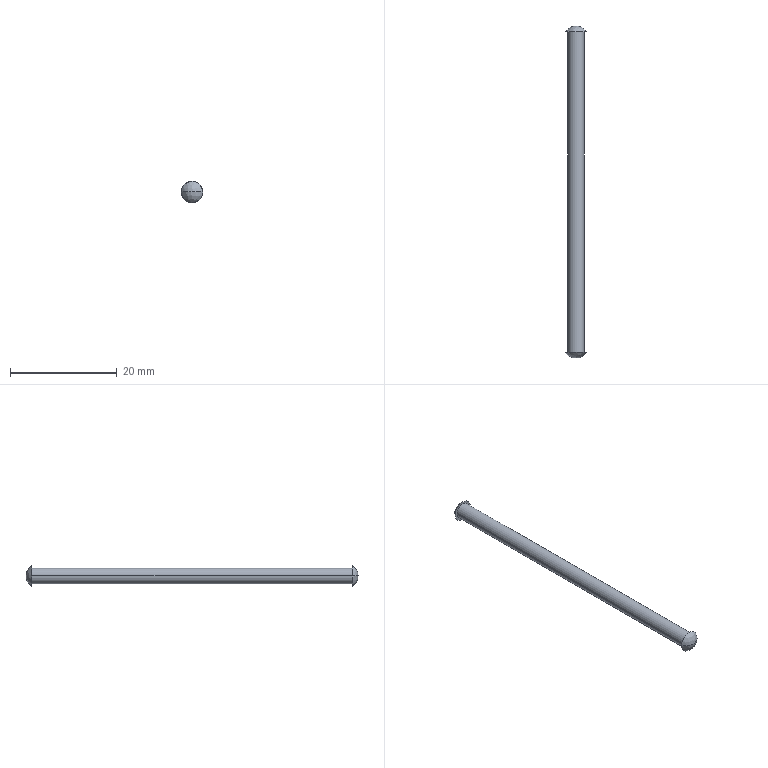Part | STEP file | Second B-1027-14 Shaft Part | 1 solid | 7 faces | box 4 x 62.171 x 4 mm | volume 439.342 mm3 | spline 3 | cylinder 2 | plane 2 | commonest cylinder face diameters 3 x2
STEP:
#1=CARTESIAN_POINT('',(-2.,-30.,0.));
#2=VERTEX_POINT('',#1);
#3=CARTESIAN_POINT('',(2.,-30.,0.));
#4=VERTEX_POINT('',#3);
#5=CARTESIAN_POINT('',(-2.,-30.,0.));
#6=CARTESIAN_POINT('',(-2.,-30.,-0.1321));
#7=CARTESIAN_POINT('',(-1.987,-30.,-0.262));
#8=CARTESIAN_POINT('',(-1.936,-30.,-0.5176));
#9=CARTESIAN_POINT('',(-1.898,-30.,-0.6446));
#10=CARTESIAN_POINT('',(-1.797,-30.,-0.8868));
#11=CARTESIAN_POINT('',(-1.736,-30.,-1.002));
#12=CARTESIAN_POINT('',(-1.591,-30.,-1.219));
#13=CARTESIAN_POINT('',(-1.506,-30.,-1.322));
#14=CARTESIAN_POINT('',(-1.23,-30.,-1.599));
#15=CARTESIAN_POINT('',(-1.007,-30.,-1.748));
#16=CARTESIAN_POINT('',(-0.5253,-30.,-1.947));
#17=CARTESIAN_POINT('',(-0.2622,-30.,-2.));
#18=CARTESIAN_POINT('',(0.1291,-30.,-2.));
#19=CARTESIAN_POINT('',(0.2615,-30.,-1.987));
#20=CARTESIAN_POINT('',(0.518,-30.,-1.936));
#21=CARTESIAN_POINT('',(0.6427,-30.,-1.898));
#22=CARTESIAN_POINT('',(0.8848,-30.,-1.798));
#23=CARTESIAN_POINT('',(1.002,-30.,-1.736));
#24=CARTESIAN_POINT('',(1.219,-30.,-1.591));
#25=CARTESIAN_POINT('',(1.32,-30.,-1.509));
#26=CARTESIAN_POINT('',(1.507,-30.,-1.322));
#27=CARTESIAN_POINT('',(1.59,-30.,-1.221));
#28=CARTESIAN_POINT('',(1.734,-30.,-1.004));
#29=CARTESIAN_POINT('',(1.797,-30.,-0.8875));
#30=CARTESIAN_POINT('',(1.898,-30.,-0.6451));
#31=CARTESIAN_POINT('',(1.935,-30.,-0.5205));
#32=CARTESIAN_POINT('',(1.987,-30.,-0.2643));
#33=CARTESIAN_POINT('',(2.,-30.,-0.1321));
#34=CARTESIAN_POINT('',(2.,-30.,0.));
#35=B_SPLINE_CURVE_WITH_KNOTS('',3,(#5,#6,#7,#8,#9,#10,#11,#12,#13,#14,#15,#16,#17,#18,#19,#20,#21,#22,#23,#24,#25,#26,#27,#28,#29,#30,#31,#32,#33,#34),.UNSPECIFIED.,.F.,.F.,(4,2,2,2,2,2,2,2,2,2,2,2,2,2,4),(0.,0.0003907,0.0007815,0.001172,0.001563,0.002344,0.003126,0.003517,0.003907,0.004298,0.004689,0.005079,0.00547,0.005861,0.006252),.UNSPECIFIED.);
#36=EDGE_CURVE('',#2,#4,#35,.T.);
#37=ORIENTED_EDGE('',*,*,#36,.T.);
#38=CARTESIAN_POINT('',(0.,-28.732,0.));
#39=DIRECTION('',(0.,0.,-1.));
#40=DIRECTION('',(1.,0.,0.));
#41=AXIS2_PLACEMENT_3D('',#38,#39,#40);
#42=CIRCLE('',#41,2.368);
#43=EDGE_CURVE('',#4,#2,#42,.T.);
#44=ORIENTED_EDGE('',*,*,#43,.T.);
#45=EDGE_LOOP('',(#37,#44));
#46=FACE_OUTER_BOUND('',#45,.T.);
#47=CARTESIAN_POINT('',(2.015,-29.976,0.));
#48=CARTESIAN_POINT('',(2.015,-29.976,-0.4398));
#49=CARTESIAN_POINT('',(2.015,-29.762,-0.8242));
#50=CARTESIAN_POINT('',(2.015,-29.389,-1.056));
#51=CARTESIAN_POINT('',(0.9827,-31.648,0.));
#52=CARTESIAN_POINT('',(0.9827,-31.648,-1.031));
#53=CARTESIAN_POINT('',(0.9827,-31.147,-1.932));
#54=CARTESIAN_POINT('',(0.9827,-30.272,-2.477));
#55=CARTESIAN_POINT('',(-0.9827,-31.648,0.));
#56=CARTESIAN_POINT('',(-0.9827,-31.648,-1.031));
#57=CARTESIAN_POINT('',(-0.9827,-31.147,-1.932));
#58=CARTESIAN_POINT('',(-0.9827,-30.272,-2.477));
#59=CARTESIAN_POINT('',(-2.015,-29.976,0.));
#60=CARTESIAN_POINT('',(-2.015,-29.976,-0.4398));
#61=CARTESIAN_POINT('',(-2.015,-29.762,-0.8242));
#62=CARTESIAN_POINT('',(-2.015,-29.389,-1.056));
#63=(BOUNDED_SURFACE()B_SPLINE_SURFACE(3,3,((#47,#48,#49,#50),(#51,#52,#53,#54),(#55,#56,#57,#58),(#59,#60,#61,#62)),.UNSPECIFIED.,.F.,.F.,.F.)B_SPLINE_SURFACE_WITH_KNOTS((4,4),(4,4),(0.,1.),(0.,1.),.UNSPECIFIED.)GEOMETRIC_REPRESENTATION_ITEM()RATIONAL_B_SPLINE_SURFACE(((1.,0.916,0.916,1.),(0.6835,0.6261,0.6261,0.6835),(0.6835,0.6261,0.6261,0.6835),(1.,0.916,0.916,1.)))REPRESENTATION_ITEM('')SURFACE());
#64=ADVANCED_FACE('',(#46),#63,.T.);
#65=CARTESIAN_POINT('',(-1.5,-30.,0.));
#66=VERTEX_POINT('',#65);
#67=CARTESIAN_POINT('',(1.5,-30.,0.));
#68=VERTEX_POINT('',#67);
#69=CARTESIAN_POINT('',(0.,-30.,0.));
#70=DIRECTION('',(0.,1.,0.));
#71=DIRECTION('',(-1.,0.,0.));
#72=AXIS2_PLACEMENT_3D('',#69,#70,#71);
#73=CIRCLE('',#72,1.5);
#74=EDGE_CURVE('',#66,#68,#73,.T.);
#75=ORIENTED_EDGE('',*,*,#74,.T.);
#76=CARTESIAN_POINT('',(1.5,30.,0.));
#77=VERTEX_POINT('',#76);
#78=CARTESIAN_POINT('',(1.5,31.1,0.));
#79=DIRECTION('',(0.,1.,0.));
#80=VECTOR('',#79,1000.);
#81=LINE('',#78,#80);
#82=EDGE_CURVE('',#68,#77,#81,.T.);
#83=ORIENTED_EDGE('',*,*,#82,.T.);
#84=CARTESIAN_POINT('',(-1.5,30.,0.));
#85=VERTEX_POINT('',#84);
#86=CARTESIAN_POINT('',(0.,30.,0.));
#87=DIRECTION('',(0.,-1.,0.));
#88=DIRECTION('',(-1.,0.,0.));
#89=AXIS2_PLACEMENT_3D('',#86,#87,#88);
#90=CIRCLE('',#89,1.5);
#91=EDGE_CURVE('',#77,#85,#90,.T.);
#92=ORIENTED_EDGE('',*,*,#91,.T.);
#93=CARTESIAN_POINT('',(-1.5,31.1,0.));
#94=DIRECTION('',(0.,1.,0.));
#95=VECTOR('',#94,1000.);
#96=LINE('',#93,#95);
#97=EDGE_CURVE('',#66,#85,#96,.T.);
#98=ORIENTED_EDGE('',*,*,#97,.F.);
#99=EDGE_LOOP('',(#75,#83,#92,#98));
#100=FACE_OUTER_BOUND('',#99,.T.);
#101=CARTESIAN_POINT('',(0.,31.1,0.));
#102=DIRECTION('',(0.,1.,0.));
#103=DIRECTION('',(-1.,0.,0.));
#104=AXIS2_PLACEMENT_3D('',#101,#102,#103);
#105=CYLINDRICAL_SURFACE('',#104,1.5);
#106=ADVANCED_FACE('',(#100),#105,.T.);
#107=ORIENTED_EDGE('',*,*,#82,.F.);
#108=CARTESIAN_POINT('',(0.,-30.,0.));
#109=DIRECTION('',(0.,1.,0.));
#110=DIRECTION('',(-1.,0.,0.));
#111=AXIS2_PLACEMENT_3D('',#108,#109,#110);
#112=CIRCLE('',#111,1.5);
#113=EDGE_CURVE('',#68,#66,#112,.T.);
#114=ORIENTED_EDGE('',*,*,#113,.T.);
#115=ORIENTED_EDGE('',*,*,#97,.T.);
#116=CARTESIAN_POINT('',(0.,30.,0.));
#117=DIRECTION('',(0.,-1.,0.));
#118=DIRECTION('',(-1.,0.,0.));
#119=AXIS2_PLACEMENT_3D('',#116,#117,#118);
#120=CIRCLE('',#119,1.5);
#121=EDGE_CURVE('',#85,#77,#120,.T.);
#122=ORIENTED_EDGE('',*,*,#121,.T.);
#123=EDGE_LOOP('',(#107,#114,#115,#122));
#124=FACE_OUTER_BOUND('',#123,.T.);
#125=CARTESIAN_POINT('',(0.,31.1,0.));
#126=DIRECTION('',(0.,1.,0.));
#127=DIRECTION('',(-1.,0.,0.));
#128=AXIS2_PLACEMENT_3D('',#125,#126,#127);
#129=CYLINDRICAL_SURFACE('',#128,1.5);
#130=ADVANCED_FACE('',(#124),#129,.T.);
#131=ORIENTED_EDGE('',*,*,#121,.F.);
#132=ORIENTED_EDGE('',*,*,#91,.F.);
#133=EDGE_LOOP('',(#131,#132));
#134=FACE_BOUND('',#133,.T.);
#135=CARTESIAN_POINT('',(2.,30.,0.));
#136=VERTEX_POINT('',#135);
#137=CARTESIAN_POINT('',(-2.,30.,0.));
#138=VERTEX_POINT('',#137);
#139=CARTESIAN_POINT('',(2.,30.,0.));
#140=CARTESIAN_POINT('',(2.,30.,-0.1321));
#141=CARTESIAN_POINT('',(1.987,30.,-0.262));
#142=CARTESIAN_POINT('',(1.936,30.,-0.5176));
#143=CARTESIAN_POINT('',(1.898,30.,-0.6446));
#144=CARTESIAN_POINT('',(1.797,30.,-0.8868));
#145=CARTESIAN_POINT('',(1.736,30.,-1.002));
#146=CARTESIAN_POINT('',(1.591,30.,-1.219));
#147=CARTESIAN_POINT('',(1.506,30.,-1.322));
#148=CARTESIAN_POINT('',(1.23,30.,-1.599));
#149=CARTESIAN_POINT('',(1.007,30.,-1.748));
#150=CARTESIAN_POINT('',(0.5253,30.,-1.947));
#151=CARTESIAN_POINT('',(0.2622,30.,-2.));
#152=CARTESIAN_POINT('',(-0.1291,30.,-2.));
#153=CARTESIAN_POINT('',(-0.2615,30.,-1.987));
#154=CARTESIAN_POINT('',(-0.518,30.,-1.936));
#155=CARTESIAN_POINT('',(-0.6427,30.,-1.898));
#156=CARTESIAN_POINT('',(-0.8848,30.,-1.798));
#157=CARTESIAN_POINT('',(-1.002,30.,-1.736));
#158=CARTESIAN_POINT('',(-1.219,30.,-1.591));
#159=CARTESIAN_POINT('',(-1.32,30.,-1.509));
#160=CARTESIAN_POINT('',(-1.507,30.,-1.322));
#161=CARTESIAN_POINT('',(-1.59,30.,-1.221));
#162=CARTESIAN_POINT('',(-1.734,30.,-1.004));
#163=CARTESIAN_POINT('',(-1.797,30.,-0.8875));
#164=CARTESIAN_POINT('',(-1.898,30.,-0.6451));
#165=CARTESIAN_POINT('',(-1.935,30.,-0.5205));
#166=CARTESIAN_POINT('',(-1.987,30.,-0.2643));
#167=CARTESIAN_POINT('',(-2.,30.,-0.1321));
#168=CARTESIAN_POINT('',(-2.,30.,0.));
#169=B_SPLINE_CURVE_WITH_KNOTS('',3,(#139,#140,#141,#142,#143,#144,#145,#146,#147,#148,#149,#150,#151,#152,#153,#154,#155,#156,#157,#158,#159,#160,#161,#162,#163,#164,#165,#166,#167,#168),.UNSPECIFIED.,.F.,.F.,(4,2,2,2,2,2,2,2,2,2,2,2,2,2,4),(0.,0.0003907,0.0007815,0.001172,0.001563,0.002344,0.003126,0.003517,0.003907,0.004298,0.004689,0.005079,0.00547,0.005861,0.006252),.UNSPECIFIED.);
#170=EDGE_CURVE('',#136,#138,#169,.T.);
#171=ORIENTED_EDGE('',*,*,#170,.F.);
#172=CARTESIAN_POINT('',(-2.,30.,0.));
#173=CARTESIAN_POINT('',(-2.,30.,0.1321));
#174=CARTESIAN_POINT('',(-1.987,30.,0.262));
#175=CARTESIAN_POINT('',(-1.936,30.,0.5176));
#176=CARTESIAN_POINT('',(-1.898,30.,0.6446));
#177=CARTESIAN_POINT('',(-1.797,30.,0.8868));
#178=CARTESIAN_POINT('',(-1.736,30.,1.002));
#179=CARTESIAN_POINT('',(-1.591,30.,1.219));
#180=CARTESIAN_POINT('',(-1.506,30.,1.322));
#181=CARTESIAN_POINT('',(-1.23,30.,1.599));
#182=CARTESIAN_POINT('',(-1.007,30.,1.748));
#183=CARTESIAN_POINT('',(-0.5253,30.,1.947));
#184=CARTESIAN_POINT('',(-0.2622,30.,2.));
#185=CARTESIAN_POINT('',(0.1291,30.,2.));
#186=CARTESIAN_POINT('',(0.2615,30.,1.987));
#187=CARTESIAN_POINT('',(0.518,30.,1.936));
#188=CARTESIAN_POINT('',(0.6427,30.,1.898));
#189=CARTESIAN_POINT('',(0.8848,30.,1.798));
#190=CARTESIAN_POINT('',(1.002,30.,1.736));
#191=CARTESIAN_POINT('',(1.219,30.,1.591));
#192=CARTESIAN_POINT('',(1.32,30.,1.509));
#193=CARTESIAN_POINT('',(1.507,30.,1.322));
#194=CARTESIAN_POINT('',(1.59,30.,1.221));
#195=CARTESIAN_POINT('',(1.734,30.,1.004));
#196=CARTESIAN_POINT('',(1.797,30.,0.8875));
#197=CARTESIAN_POINT('',(1.898,30.,0.6451));
#198=CARTESIAN_POINT('',(1.935,30.,0.5205));
#199=CARTESIAN_POINT('',(1.987,30.,0.2643));
#200=CARTESIAN_POINT('',(2.,30.,0.1321));
#201=CARTESIAN_POINT('',(2.,30.,0.));
#202=B_SPLINE_CURVE_WITH_KNOTS('',3,(#172,#173,#174,#175,#176,#177,#178,#179,#180,#181,#182,#183,#184,#185,#186,#187,#188,#189,#190,#191,#192,#193,#194,#195,#196,#197,#198,#199,#200,#201),.UNSPECIFIED.,.F.,.F.,(4,2,2,2,2,2,2,2,2,2,2,2,2,2,4),(0.006252,0.006642,0.007033,0.007424,0.007815,0.008596,0.009377,0.009768,0.01016,0.01055,0.01094,0.01133,0.01172,0.01211,0.0125),.UNSPECIFIED.);
#203=EDGE_CURVE('',#138,#136,#202,.T.);
#204=ORIENTED_EDGE('',*,*,#203,.F.);
#205=EDGE_LOOP('',(#171,#204));
#206=FACE_OUTER_BOUND('',#205,.T.);
#207=CARTESIAN_POINT('',(1.5,30.,0.));
#208=DIRECTION('',(0.,1.,0.));
#209=DIRECTION('',(-1.,0.,0.));
#210=AXIS2_PLACEMENT_3D('',#207,#208,#209);
#211=PLANE('',#210);
#212=ADVANCED_FACE('',(#134,#206),#211,.F.);
#213=ORIENTED_EDGE('',*,*,#36,.F.);
#214=CARTESIAN_POINT('',(2.,-30.,0.));
#215=CARTESIAN_POINT('',(2.,-30.,0.1321));
#216=CARTESIAN_POINT('',(1.987,-30.,0.262));
#217=CARTESIAN_POINT('',(1.936,-30.,0.5176));
#218=CARTESIAN_POINT('',(1.898,-30.,0.6446));
#219=CARTESIAN_POINT('',(1.797,-30.,0.8868));
#220=CARTESIAN_POINT('',(1.736,-30.,1.002));
#221=CARTESIAN_POINT('',(1.591,-30.,1.219));
#222=CARTESIAN_POINT('',(1.506,-30.,1.322));
#223=CARTESIAN_POINT('',(1.23,-30.,1.599));
#224=CARTESIAN_POINT('',(1.007,-30.,1.748));
#225=CARTESIAN_POINT('',(0.5253,-30.,1.947));
#226=CARTESIAN_POINT('',(0.2622,-30.,2.));
#227=CARTESIAN_POINT('',(-0.1291,-30.,2.));
#228=CARTESIAN_POINT('',(-0.2615,-30.,1.987));
#229=CARTESIAN_POINT('',(-0.518,-30.,1.936));
#230=CARTESIAN_POINT('',(-0.6427,-30.,1.898));
#231=CARTESIAN_POINT('',(-0.8848,-30.,1.798));
#232=CARTESIAN_POINT('',(-1.002,-30.,1.736));
#233=CARTESIAN_POINT('',(-1.219,-30.,1.591));
#234=CARTESIAN_POINT('',(-1.32,-30.,1.509));
#235=CARTESIAN_POINT('',(-1.507,-30.,1.322));
#236=CARTESIAN_POINT('',(-1.59,-30.,1.221));
#237=CARTESIAN_POINT('',(-1.734,-30.,1.004));
#238=CARTESIAN_POINT('',(-1.797,-30.,0.8875));
#239=CARTESIAN_POINT('',(-1.898,-30.,0.6451));
#240=CARTESIAN_POINT('',(-1.935,-30.,0.5205));
#241=CARTESIAN_POINT('',(-1.987,-30.,0.2643));
#242=CARTESIAN_POINT('',(-2.,-30.,0.1321));
#243=CARTESIAN_POINT('',(-2.,-30.,0.));
#244=B_SPLINE_CURVE_WITH_KNOTS('',3,(#214,#215,#216,#217,#218,#219,#220,#221,#222,#223,#224,#225,#226,#227,#228,#229,#230,#231,#232,#233,#234,#235,#236,#237,#238,#239,#240,#241,#242,#243),.UNSPECIFIED.,.F.,.F.,(4,2,2,2,2,2,2,2,2,2,2,2,2,2,4),(0.006252,0.006642,0.007033,0.007424,0.007815,0.008596,0.009377,0.009768,0.01016,0.01055,0.01094,0.01133,0.01172,0.01211,0.0125),.UNSPECIFIED.);
#245=EDGE_CURVE('',#4,#2,#244,.T.);
#246=ORIENTED_EDGE('',*,*,#245,.F.);
#247=EDGE_LOOP('',(#213,#246));
#248=FACE_OUTER_BOUND('',#247,.T.);
#249=ORIENTED_EDGE('',*,*,#74,.F.);
#250=ORIENTED_EDGE('',*,*,#113,.F.);
#251=EDGE_LOOP('',(#249,#250));
#252=FACE_BOUND('',#251,.T.);
#253=CARTESIAN_POINT('',(1.5,-30.,0.));
#254=DIRECTION('',(0.,-1.,0.));
#255=DIRECTION('',(1.,0.,0.));
#256=AXIS2_PLACEMENT_3D('',#253,#254,#255);
#257=PLANE('',#256);
#258=ADVANCED_FACE('',(#248,#252),#257,.F.);
#259=ORIENTED_EDGE('',*,*,#170,.T.);
#260=ORIENTED_EDGE('',*,*,#203,.T.);
#261=EDGE_LOOP('',(#259,#260));
#262=FACE_OUTER_BOUND('',#261,.T.);
#263=CARTESIAN_POINT('',(2.015,29.382,-1.06));
#264=CARTESIAN_POINT('',(2.015,30.266,-0.5184));
#265=CARTESIAN_POINT('',(2.015,30.266,0.5184));
#266=CARTESIAN_POINT('',(2.015,29.382,1.06));
#267=CARTESIAN_POINT('',(0.9827,30.257,-2.486));
#268=CARTESIAN_POINT('',(0.9827,32.329,-1.215));
#269=CARTESIAN_POINT('',(0.9827,32.329,1.215));
#270=CARTESIAN_POINT('',(0.9827,30.257,2.486));
#271=CARTESIAN_POINT('',(-0.9827,30.257,-2.486));
#272=CARTESIAN_POINT('',(-0.9827,32.329,-1.215));
#273=CARTESIAN_POINT('',(-0.9827,32.329,1.215));
#274=CARTESIAN_POINT('',(-0.9827,30.257,2.486));
#275=CARTESIAN_POINT('',(-2.015,29.382,-1.06));
#276=CARTESIAN_POINT('',(-2.015,30.266,-0.5184));
#277=CARTESIAN_POINT('',(-2.015,30.266,0.5184));
#278=CARTESIAN_POINT('',(-2.015,29.382,1.06));
#279=(BOUNDED_SURFACE()B_SPLINE_SURFACE(3,3,((#263,#264,#265,#266),(#267,#268,#269,#270),(#271,#272,#273,#274),(#275,#276,#277,#278)),.UNSPECIFIED.,.F.,.F.,.F.)B_SPLINE_SURFACE_WITH_KNOTS((4,4),(4,4),(0.,1.),(0.,1.),.UNSPECIFIED.)GEOMETRIC_REPRESENTATION_ITEM()RATIONAL_B_SPLINE_SURFACE(((1.,0.6819,0.6819,1.),(0.6835,0.4661,0.4661,0.6835),(0.6835,0.4661,0.4661,0.6835),(1.,0.6819,0.6819,1.)))REPRESENTATION_ITEM('')SURFACE());
#280=ADVANCED_FACE('',(#262),#279,.T.);
#281=ORIENTED_EDGE('',*,*,#43,.F.);
#282=ORIENTED_EDGE('',*,*,#245,.T.);
#283=EDGE_LOOP('',(#281,#282));
#284=FACE_OUTER_BOUND('',#283,.T.);
#285=CARTESIAN_POINT('',(2.015,-29.389,1.056));
#286=CARTESIAN_POINT('',(2.015,-29.762,0.8242));
#287=CARTESIAN_POINT('',(2.015,-29.976,0.4398));
#288=CARTESIAN_POINT('',(2.015,-29.976,0.));
#289=CARTESIAN_POINT('',(0.9827,-30.272,2.477));
#290=CARTESIAN_POINT('',(0.9827,-31.147,1.932));
#291=CARTESIAN_POINT('',(0.9827,-31.648,1.031));
#292=CARTESIAN_POINT('',(0.9827,-31.648,0.));
#293=CARTESIAN_POINT('',(-0.9827,-30.272,2.477));
#294=CARTESIAN_POINT('',(-0.9827,-31.147,1.932));
#295=CARTESIAN_POINT('',(-0.9827,-31.648,1.031));
#296=CARTESIAN_POINT('',(-0.9827,-31.648,0.));
#297=CARTESIAN_POINT('',(-2.015,-29.389,1.056));
#298=CARTESIAN_POINT('',(-2.015,-29.762,0.8242));
#299=CARTESIAN_POINT('',(-2.015,-29.976,0.4398));
#300=CARTESIAN_POINT('',(-2.015,-29.976,0.));
#301=(BOUNDED_SURFACE()B_SPLINE_SURFACE(3,3,((#285,#286,#287,#288),(#289,#290,#291,#292),(#293,#294,#295,#296),(#297,#298,#299,#300)),.UNSPECIFIED.,.F.,.F.,.F.)B_SPLINE_SURFACE_WITH_KNOTS((4,4),(4,4),(0.,1.),(0.,1.),.UNSPECIFIED.)GEOMETRIC_REPRESENTATION_ITEM()RATIONAL_B_SPLINE_SURFACE(((1.,0.916,0.916,1.),(0.6835,0.6261,0.6261,0.6835),(0.6835,0.6261,0.6261,0.6835),(1.,0.916,0.916,1.)))REPRESENTATION_ITEM('')SURFACE());
#302=ADVANCED_FACE('',(#284),#301,.T.);
#303=CLOSED_SHELL('',(#64,#106,#130,#212,#258,#280,#302));
#304=MANIFOLD_SOLID_BREP('',#303);
#305=CARTESIAN_POINT('',(0.,0.,0.));
#306=DIRECTION('',(0.,0.,1.));
#307=DIRECTION('',(1.,0.,0.));
#308=AXIS2_PLACEMENT_3D('',#305,#306,#307);
#309=(LENGTH_UNIT()NAMED_UNIT(*)SI_UNIT(.MILLI.,.METRE.));
#310=UNCERTAINTY_MEASURE_WITH_UNIT(LENGTH_MEASURE(0.00001),#309,'','');
#311=(NAMED_UNIT(*)PLANE_ANGLE_UNIT()SI_UNIT($,.RADIAN.));
#312=(NAMED_UNIT(*)SI_UNIT($,.STERADIAN.)SOLID_ANGLE_UNIT());
#313=(GEOMETRIC_REPRESENTATION_CONTEXT(3)GLOBAL_UNCERTAINTY_ASSIGNED_CONTEXT((#310))GLOBAL_UNIT_ASSIGNED_CONTEXT((#309,#311,#312))REPRESENTATION_CONTEXT('',''));
#314=ADVANCED_BREP_SHAPE_REPRESENTATION('',(#304,#308),#313);